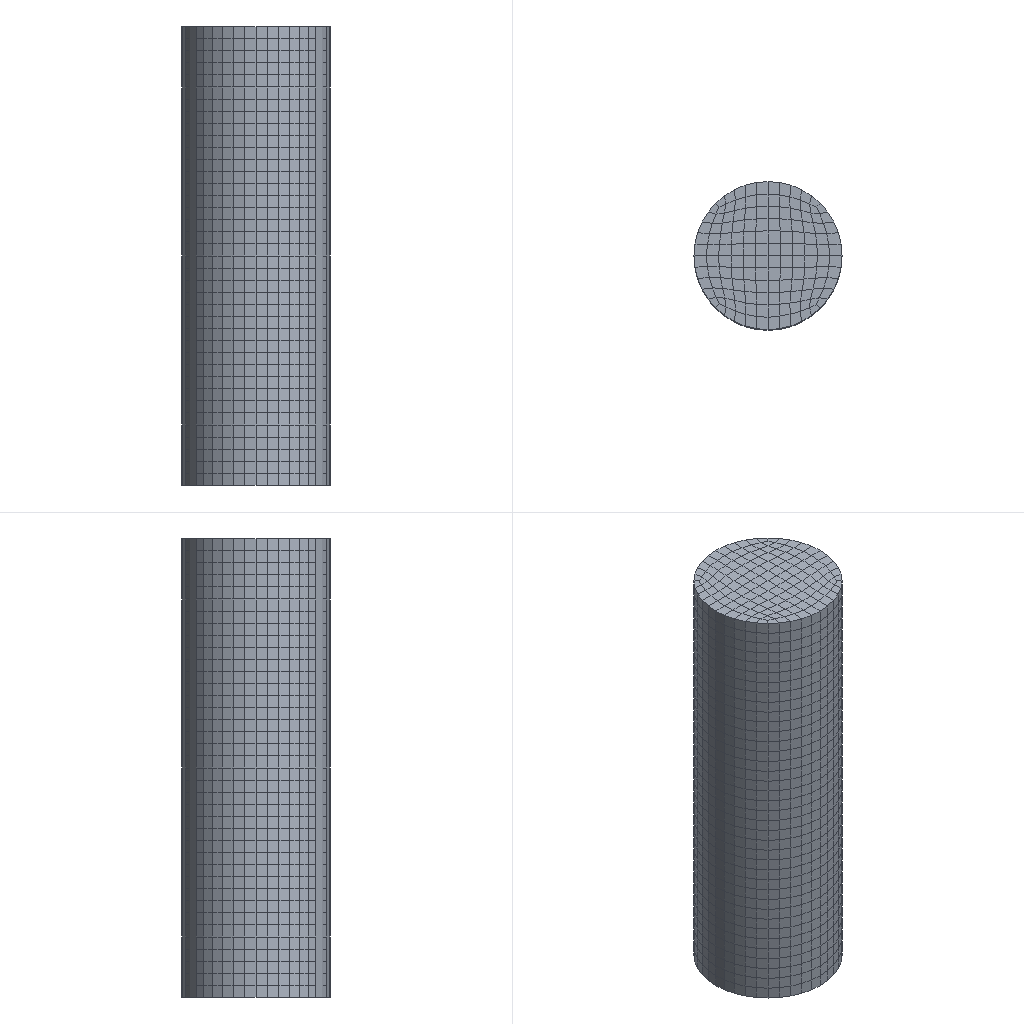Simulation study | abaqus
Set-up summary:
category,name,step,type,value,unit,region
solver,abaqus
solver,version,,,Abaqus/Standard 3DEXPERIENCE R2017x
units,not stated in the deck,,not stated
analysis,deck,,static,static
load_step,Step-1,Step-1,static,nlgeom=False
load_step,Step-2,Step-2,static,nlgeom=False
contact,interactions,,,general=0 pairs=1 ties=0
load_step,requested,,,2
mesh,nodes,,,7839
mesh,elements,,,6840
element_type,S4R,,shell,1520
element_type,C3D8R,,solid,5320
load,load commands in deck,,count,1
bc,support commands in deck,,count,13
material,H,,in results
material,S,,in results
check,setup vs results,,match,"per instance, exact: element labels, types and connectivity; labels of the nodes the elements use; coordinates of those nodes at SINGLE_PRECISION in 1 of 2 instance(s)"
Abaqus input file, long lists of numbers shortened:
*Heading
** Job name: Job-10 Model name: Model-1-Copy-Copy
** Generated by: Abaqus/CAE 2017
*Preprint, echo=NO, model=NO, history=NO, contact=NO
**
** PARTS
**
*Part, name=h
*Node
      1,           0.,           0.,         0.75
      2,           0., -0.121,         0.75
** (6277 more lines like these left out)
*Element, type=C3D8R
   1,  518,  519, 2929, 2641,   11,   12,  309,  308
   2,  519,  520, 2930, 2929,   12,   13,  310,  309
** (5318 more lines like these left out)
*Nset, nset=_PickedSet5, internal, generate
    1,  6279,     1
*Elset, elset=_PickedSet5, internal, generate
    1,  5320,     1
** Section: h
*Solid Section, elset=_PickedSet5, material=h
,
*End Part
**
*Part, name=ke
*Node
      1,           0., -0.121,           0.
      2,           0., -0.121,         0.75
** (1558 more lines like these left out)
*Element, type=S4R
  1,   1,   9, 229, 100
  2,   9,  10, 230, 229
** (1518 more lines like these left out)
*Nset, nset=Set-1, generate
    1,  1560,     1
*Elset, elset=Set-1, generate
    1,  1520,     1
** Section: Section-ke
*Shell Section, elset=Set-1, material=s, temperature=9, offset=-0.5
0.004, 9
*End Part
**
**
** ASSEMBLY
**
*Assembly, name=Assembly
**
*Instance, name=h-1, part=h
*End Instance
**
*Instance, name=ke-1, part=ke
*End Instance
**
*Node
      1,  -6.9388939e-18,  -7.40911299e-18,         0.75
*Node
      2,  2.08166817e-17,  -7.40911299e-18,           0.
*Nset, nset=Set-2, instance=h-1, generate
    1,  6279,     1
*Nset, nset=Set-2, instance=ke-1
 1, 2
*Elset, elset=Set-2, instance=h-1, generate
    1,  5320,     1
*Nset, nset=Set-3, instance=h-1, generate
    1,  6279,     1
*Nset, nset=Set-3, instance=ke-1, generate
    1,  1560,     1
*Elset, elset=Set-3, instance=h-1, generate
    1,  5320,     1
*Elset, elset=Set-3, instance=ke-1, generate
    1,  1520,     1
*Nset, nset=Set-4
 1,
*Nset, nset=Set-5
 2,
*Nset, nset=Set-9, instance=h-1, generate
    1,  6279,     1
*Nset, nset=Set-9, instance=ke-1, generate
    1,  1560,     1
*Elset, elset=Set-9, instance=h-1, generate
    1,  5320,     1
*Elset, elset=Set-9, instance=ke-1, generate
    1,  1520,     1
*Nset, nset=Set-10, instance=h-1, generate
    1,  6279,     1
*Nset, nset=Set-10, instance=ke-1, generate
    1,  1560,     1
*Elset, elset=Set-10, instance=h-1, generate
    1,  5320,     1
*Elset, elset=Set-10, instance=ke-1, generate
    1,  1520,     1
*Nset, nset=Set-11, instance=h-1, generate
    1,  6279,     1
*Nset, nset=Set-11, instance=ke-1, generate
    1,  1560,     1
*Elset, elset=Set-11, instance=h-1, generate
    1,  5320,     1
*Elset, elset=Set-11, instance=ke-1, generate
    1,  1520,     1
*Nset, nset=Set-19, instance=h-1, generate
    1,  6279,     1
*Nset, nset=Set-19, instance=ke-1, generate
    1,  1560,     1
*Elset, elset=Set-19, instance=h-1, generate
    1,  5320,     1
*Elset, elset=Set-19, instance=ke-1, generate
    1,  1520,     1
*Nset, nset=Set-20, instance=h-1
    1,    2,    3,    4,    5,    6,    7,    8,    9,   10,   11,   12,   13,   14,   15,   16
   17,   18,   19,   20,   21,   22,   23,   24,   25,   26,   27,   28,   29,   30,   31,   32
** (59 more lines like these left out)
*Nset, nset=Set-20, instance=ke-1, generate
    1,  1560,     1
*Elset, elset=Set-20, instance=h-1
    1,    2,    3,    4,    5,   10,   15,   20,   25,   26,   27,   28,   29,   30,   35,   40
   45,   50,   51,   52,   53,   54,   55,   60,   65,   70,   75,   76,   77,   78,   79,   80
** (103 more lines like these left out)
*Elset, elset=Set-20, instance=ke-1, generate
    1,  1520,     1
*Nset, nset=Set-21, instance=h-1
    1,    2,    3,    4,    5,    6,    7,    8,    9,   10,   11,   12,   13,   14,   15,   16
   17,   18,   19,   20,   21,   22,   23,   24,   25,   26,   27,   28,   29,   30,   31,   32
** (64 more lines like these left out)
*Elset, elset=Set-21, instance=h-1
    1,    2,    3,    4,    5,   10,   15,   20,   25,   26,   27,   28,   29,   30,   35,   40
   45,   50,   51,   52,   53,   54,   55,   60,   65,   70,   75,   76,   77,   78,   79,   80
** (107 more lines like these left out)
*Nset, nset=Set-22, instance=h-1, generate
    1,  6279,     1
*Nset, nset=Set-22, instance=ke-1, generate
    1,  1560,     1
*Elset, elset=Set-22, instance=h-1, generate
    1,  5320,     1
*Elset, elset=Set-22, instance=ke-1, generate
    1,  1520,     1
*Nset, nset=Set-23, instance=h-1, generate
    1,  6279,     1
*Elset, elset=Set-23, instance=h-1, generate
    1,  5320,     1
*Nset, nset=Set-24, instance=h-1
    1,    2,    3,    4,    5,    6,    7,    8,    9,   10,   11,   12,   13,   14,   15,   16
   17,   18,   19,   20,   21,   22,   23,   24,   25,   26,   27,   28,   29,   30,   31,   32
** (64 more lines like these left out)
*Elset, elset=Set-24, instance=h-1
    1,    2,    3,    4,    5,   10,   15,   20,   25,   26,   27,   28,   29,   30,   35,   40
   45,   50,   51,   52,   53,   54,   55,   60,   65,   70,   75,   76,   77,   78,   79,   80
** (107 more lines like these left out)
*Nset, nset=Set-25, instance=h-1, generate
    1,  6279,     1
*Elset, elset=Set-25, instance=h-1, generate
    1,  5320,     1
*Nset, nset=Set-26, instance=h-1
    1,    2,    3,    4,    5,    6,    7,    8,    9,   10,   11,   12,   13,   14,   15,   16
   17,   18,   19,   20,   21,   22,   23,   24,   25,   26,   27,   28,   29,   30,   31,   32
** (64 more lines like these left out)
*Nset, nset=Set-26, instance=ke-1, generate
    1,  1560,     1
*Elset, elset=Set-26, instance=h-1
    1,    2,    3,    4,    5,   10,   15,   20,   25,   26,   27,   28,   29,   30,   35,   40
   45,   50,   51,   52,   53,   54,   55,   60,   65,   70,   75,   76,   77,   78,   79,   80
** (107 more lines like these left out)
*Elset, elset=Set-26, instance=ke-1, generate
    1,  1520,     1
*Nset, nset=Set-27, instance=h-1, generate
    1,  6279,     1
*Elset, elset=Set-27, instance=h-1, generate
    1,  5320,     1
*Nset, nset=Set-28, instance=h-1, generate
    1,  6279,     1
*Elset, elset=Set-28, instance=h-1, generate
    1,  5320,     1
*Nset, nset=Set-29, instance=h-1
    1,    2,    3,    4,    5,    6,    7,    8,    9,   10,   11,   12,   13,   14,   15,   16
   17,   18,   19,   20,   21,   22,   23,   24,   25,   26,   27,   28,   29,   30,   31,   32
** (147 more lines like these left out)
*Elset, elset=Set-29, instance=h-1
    1,    2,    3,    4,    5,   10,   15,   20,   25,   26,   27,   28,   29,   30,   35,   40
   45,   50,   51,   52,   53,   54,   55,   60,   65,   70,   75,   76,   77,   78,   79,   80
** (179 more lines like these left out)
*Nset, nset=Set-30, instance=h-1, generate
    1,  6279,     1
*Nset, nset=Set-30, instance=ke-1, generate
    1,  1560,     1
*Elset, elset=Set-30, instance=h-1, generate
    1,  5320,     1
*Elset, elset=Set-30, instance=ke-1, generate
    1,  1520,     1
*Nset, nset=Set-31, instance=h-1, generate
    1,  6279,     1
*Nset, nset=Set-31, instance=ke-1, generate
    1,  1560,     1
*Elset, elset=Set-31, instance=h-1, generate
    1,  5320,     1
*Elset, elset=Set-31, instance=ke-1, generate
    1,  1520,     1
*Nset, nset=Set-32, instance=h-1
    1,    2,    3,    4,    5,    6,    7,    8,    9,   10,   11,   12,   13,   14,   15,   16
   17,   18,   19,   20,   21,   22,   23,   24,   25,   26,   27,   28,   29,   30,   31,   32
** (146 more lines like these left out)
*Nset, nset=Set-32, instance=ke-1, generate
    1,  1560,     1
*Elset, elset=Set-32, instance=h-1
    1,    2,    3,    4,    5,   10,   15,   20,   25,   26,   27,   28,   29,   30,   35,   40
   45,   50,   51,   52,   53,   54,   55,   60,   65,   70,   75,   76,   77,   78,   79,   80
** (163 more lines like these left out)
*Elset, elset=Set-32, instance=ke-1, generate
    1,  1520,     1
*Nset, nset=Set-33, instance=h-1, generate
    1,  6279,     1
*Elset, elset=Set-33, instance=h-1, generate
    1,  5320,     1
*Nset, nset=Set-37, instance=h-1, generate
    1,  6279,     1
*Elset, elset=Set-37, instance=h-1, generate
    1,  5320,     1
*Nset, nset=Set-38, instance=h-1, generate
    1,  6279,     1
*Elset, elset=Set-38, instance=h-1, generate
    1,  5320,     1
*Nset, nset=Set-39, instance=h-1, generate
    1,  6279,     1
*Nset, nset=Set-39, instance=ke-1, generate
    1,  1560,     1
*Elset, elset=Set-39, instance=h-1, generate
    1,  5320,     1
*Elset, elset=Set-39, instance=ke-1, generate
    1,  1520,     1
*Nset, nset=all, instance=h-1
    1,    2,    3,    4,    5,    6,    7,    8,    9,   10,   11,   12,   13,   14,   15,   16
   17,   18,   19,   20,   21,   22,   23,   24,   25,   26,   27,   28,   29,   30,   31,   32
** (147 more lines like these left out)
*Nset, nset=all, instance=ke-1, generate
    1,  1560,     1
*Elset, elset=all, instance=h-1
    1,    2,    3,    4,    5,   10,   15,   20,   25,   26,   27,   28,   29,   30,   35,   40
   45,   50,   51,   52,   53,   54,   55,   60,   65,   70,   75,   76,   77,   78,   79,   80
** (179 more lines like these left out)
*Elset, elset=all, instance=ke-1, generate
    1,  1520,     1
*Nset, nset=r1, instance=h-1
    1,    2,    3,    8,   10,   11,   12,   13,   14,   15,   16,   17,   18,   19,   20,   58
   59,   60,   61,   62,   63,   64,   65,   66,  211,  212,  213,  214,  215,  216,  217,  218
** (9 more lines like these left out)
*Nset, nset=r1, instance=ke-1
   2,   3,   5,   8,  46,  47,  48,  49,  50,  51,  52,  53,  54, 147, 148, 149
 150, 151, 152, 153, 154, 155, 202, 203, 204, 205, 206, 207, 208, 209, 210, 211
** (1 more lines like these left out)
*Nset, nset=r2, instance=h-1
    4,    5,    6,    7,    9,  141,  142,  143,  144,  145,  146,  147,  148,  149,  150,  151
  152,  153,  154,  155,  156,  157,  158,  159,  160,  161,  162,  163,  164,  165,  166,  167
** (9 more lines like these left out)
*Nset, nset=r2, instance=ke-1
   1,   4,   6,   7,  92,  93,  94,  95,  96,  97,  98,  99, 100, 138, 139, 140
 141, 142, 143, 144, 145, 146, 156, 157, 158, 159, 160, 161, 162, 163, 164, 220
** (1 more lines like these left out)
*Nset, nset=t_Set-5, instance=h-1
    1,    2,    3,    8,   10,   11,   12,   13,   14,   15,   16,   17,   18,   19,   20,   58
   59,   60,   61,   62,   63,   64,   65,   66,  211,  212,  213,  214,  215,  216,  217,  218
** (9 more lines like these left out)
*Nset, nset=t_Set-5, instance=ke-1
   2,   3,   5,   8,  46,  47,  48,  49,  50,  51,  52,  53,  54, 147, 148, 149
 150, 151, 152, 153, 154, 155, 202, 203, 204, 205, 206, 207, 208, 209, 210, 211
** (1 more lines like these left out)
*Elset, elset=t_Set-5, instance=h-1
    1,    2,    3,    4,    5,    6,    7,    8,    9,   10,   11,   12,   13,   14,   15,   16
   17,   18,   19,   20,   21,   22,   23,   24,   25,  476,  477,  478,  479,  480,  571,  572
** (7 more lines like these left out)
*Elset, elset=t_Set-5, instance=ke-1
   38,   76,  114,  152,  190,  228,  266,  304,  342,  380,  381,  419,  457,  495,  533,  571
  609,  647,  685,  723,  761,  799,  837,  875,  913,  951,  989, 1027, 1065, 1103, 1178, 1216
** (1 more lines like these left out)
*Nset, nset=t_Set-7, instance=h-1
    4,    5,    6,    7,    9,  141,  142,  143,  144,  145,  146,  147,  148,  149,  150,  151
  152,  153,  154,  155,  156,  157,  158,  159,  160,  161,  162,  163,  164,  165,  166,  167
** (9 more lines like these left out)
*Nset, nset=t_Set-7, instance=ke-1
   1,   4,   6,   7,  92,  93,  94,  95,  96,  97,  98,  99, 100, 138, 139, 140
 141, 142, 143, 144, 145, 146, 156, 157, 158, 159, 160, 161, 162, 163, 164, 220
** (1 more lines like these left out)
*Elset, elset=t_Set-7, instance=h-1
  684,  703,  722,  741,  760,  779,  798,  817,  836,  855,  874,  893,  912,  931,  950,  969
  988, 1007, 1026, 1045, 1064, 1083, 1102, 1121, 1140, 1141, 1160, 1179, 1198, 1217, 1254, 1273
** (7 more lines like these left out)
*Elset, elset=t_Set-7, instance=ke-1
    1,   39,   77,  115,  153,  191,  229,  267,  305,  343,  418,  456,  494,  532,  570,  608
  646,  684,  722,  760,  798,  836,  874,  912,  950,  988, 1026, 1064, 1102, 1140, 1141, 1179
** (1 more lines like these left out)
*Nset, nset=t_Set-12, instance=h-1
    1,    2,    3,    8,   10,   11,   12,   13,   14,   15,   16,   17,   18,   19,   20,   58
   59,   60,   61,   62,   63,   64,   65,   66,  211,  212,  213,  214,  215,  216,  217,  218
** (9 more lines like these left out)
*Nset, nset=t_Set-12
 1,
*Nset, nset=t_Set-12, instance=ke-1
   2,   3,   5,   8,  46,  47,  48,  49,  50,  51,  52,  53,  54, 147, 148, 149
 150, 151, 152, 153, 154, 155, 202, 203, 204, 205, 206, 207, 208, 209, 210, 211
** (1 more lines like these left out)
*Elset, elset=t_Set-12, instance=h-1
    1,    2,    3,    4,    5,    6,    7,    8,    9,   10,   11,   12,   13,   14,   15,   16
   17,   18,   19,   20,   21,   22,   23,   24,   25,  476,  477,  478,  479,  480,  571,  572
** (7 more lines like these left out)
*Elset, elset=t_Set-12, instance=ke-1
   38,   76,  114,  152,  190,  228,  266,  304,  342,  380,  381,  419,  457,  495,  533,  571
  609,  647,  685,  723,  761,  799,  837,  875,  913,  951,  989, 1027, 1065, 1103, 1178, 1216
** (1 more lines like these left out)
*Nset, nset=t_Set-13, instance=h-1
    4,    5,    6,    7,    9,  141,  142,  143,  144,  145,  146,  147,  148,  149,  150,  151
  152,  153,  154,  155,  156,  157,  158,  159,  160,  161,  162,  163,  164,  165,  166,  167
** (9 more lines like these left out)
*Nset, nset=t_Set-13
 2,
*Nset, nset=t_Set-13, instance=ke-1
   1,   4,   6,   7,  92,  93,  94,  95,  96,  97,  98,  99, 100, 138, 139, 140
 141, 142, 143, 144, 145, 146, 156, 157, 158, 159, 160, 161, 162, 163, 164, 220
** (1 more lines like these left out)
*Elset, elset=t_Set-13, instance=h-1
  684,  703,  722,  741,  760,  779,  798,  817,  836,  855,  874,  893,  912,  931,  950,  969
  988, 1007, 1026, 1045, 1064, 1083, 1102, 1121, 1140, 1141, 1160, 1179, 1198, 1217, 1254, 1273
** (7 more lines like these left out)
*Elset, elset=t_Set-13, instance=ke-1
    1,   39,   77,  115,  153,  191,  229,  267,  305,  343,  418,  456,  494,  532,  570,  608
  646,  684,  722,  760,  798,  836,  874,  912,  950,  988, 1026, 1064, 1102, 1140, 1141, 1179
** (1 more lines like these left out)
*Nset, nset=t_Set-17, instance=h-1
    1,    2,    3,    8,   10,   11,   12,   13,   14,   15,   16,   17,   18,   19,   20,   58
   59,   60,   61,   62,   63,   64,   65,   66,  211,  212,  213,  214,  215,  216,  217,  218
** (9 more lines like these left out)
*Nset, nset=t_Set-17, instance=ke-1
   2,   3,   5,   8,  46,  47,  48,  49,  50,  51,  52,  53,  54, 147, 148, 149
 150, 151, 152, 153, 154, 155, 202, 203, 204, 205, 206, 207, 208, 209, 210, 211
** (1 more lines like these left out)
*Elset, elset=t_Set-17, instance=h-1
    1,    2,    3,    4,    5,    6,    7,    8,    9,   10,   11,   12,   13,   14,   15,   16
   17,   18,   19,   20,   21,   22,   23,   24,   25,  476,  477,  478,  479,  480,  571,  572
** (7 more lines like these left out)
*Elset, elset=t_Set-17, instance=ke-1
   38,   76,  114,  152,  190,  228,  266,  304,  342,  380,  381,  419,  457,  495,  533,  571
  609,  647,  685,  723,  761,  799,  837,  875,  913,  951,  989, 1027, 1065, 1103, 1178, 1216
** (1 more lines like these left out)
*Nset, nset=t_Set-18, instance=h-1
    4,    5,    6,    7,    9,  141,  142,  143,  144,  145,  146,  147,  148,  149,  150,  151
  152,  153,  154,  155,  156,  157,  158,  159,  160,  161,  162,  163,  164,  165,  166,  167
** (9 more lines like these left out)
*Nset, nset=t_Set-18, instance=ke-1
   1,   4,   6,   7,  92,  93,  94,  95,  96,  97,  98,  99, 100, 138, 139, 140
 141, 142, 143, 144, 145, 146, 156, 157, 158, 159, 160, 161, 162, 163, 164, 220
** (1 more lines like these left out)
*Elset, elset=t_Set-18, instance=h-1
  684,  703,  722,  741,  760,  779,  798,  817,  836,  855,  874,  893,  912,  931,  950,  969
  988, 1007, 1026, 1045, 1064, 1083, 1102, 1121, 1140, 1141, 1160, 1179, 1198, 1217, 1254, 1273
** (7 more lines like these left out)
*Elset, elset=t_Set-18, instance=ke-1
    1,   39,   77,  115,  153,  191,  229,  267,  305,  343,  418,  456,  494,  532,  570,  608
  646,  684,  722,  760,  798,  836,  874,  912,  950,  988, 1026, 1064, 1102, 1140, 1141, 1179
** (1 more lines like these left out)
*Nset, nset=t_Set-34, instance=h-1
    1,    2,    3,    8,   10,   11,   12,   13,   14,   15,   16,   17,   18,   19,   20,   58
   59,   60,   61,   62,   63,   64,   65,   66,  211,  212,  213,  214,  215,  216,  217,  218
** (9 more lines like these left out)
*Nset, nset=t_Set-34, instance=ke-1
   2,   3,   5,   8,  46,  47,  48,  49,  50,  51,  52,  53,  54, 147, 148, 149
 150, 151, 152, 153, 154, 155, 202, 203, 204, 205, 206, 207, 208, 209, 210, 211
** (1 more lines like these left out)
*Elset, elset=t_Set-34, instance=h-1
    1,    2,    3,    4,    5,    6,    7,    8,    9,   10,   11,   12,   13,   14,   15,   16
   17,   18,   19,   20,   21,   22,   23,   24,   25,  476,  477,  478,  479,  480,  571,  572
** (7 more lines like these left out)
*Elset, elset=t_Set-34, instance=ke-1
   38,   76,  114,  152,  190,  228,  266,  304,  342,  380,  381,  419,  457,  495,  533,  571
  609,  647,  685,  723,  761,  799,  837,  875,  913,  951,  989, 1027, 1065, 1103, 1178, 1216
** (1 more lines like these left out)
*Nset, nset=t_Set-35, instance=h-1
    1,    2,    3,    8,   10,   11,   12,   13,   14,   15,   16,   17,   18,   19,   20,   58
   59,   60,   61,   62,   63,   64,   65,   66,  211,  212,  213,  214,  215,  216,  217,  218
** (9 more lines like these left out)
*Nset, nset=t_Set-35, instance=ke-1
   2,   3,   5,   8,  46,  47,  48,  49,  50,  51,  52,  53,  54, 147, 148, 149
 150, 151, 152, 153, 154, 155, 202, 203, 204, 205, 206, 207, 208, 209, 210, 211
** (1 more lines like these left out)
*Elset, elset=t_Set-35, instance=h-1
    1,    2,    3,    4,    5,    6,    7,    8,    9,   10,   11,   12,   13,   14,   15,   16
   17,   18,   19,   20,   21,   22,   23,   24,   25,  476,  477,  478,  479,  480,  571,  572
** (7 more lines like these left out)
*Elset, elset=t_Set-35, instance=ke-1
   38,   76,  114,  152,  190,  228,  266,  304,  342,  380,  381,  419,  457,  495,  533,  571
  609,  647,  685,  723,  761,  799,  837,  875,  913,  951,  989, 1027, 1065, 1103, 1178, 1216
** (1 more lines like these left out)
*Nset, nset=t_Set-36, instance=h-1
    4,    5,    6,    7,    9,  141,  142,  143,  144,  145,  146,  147,  148,  149,  150,  151
  152,  153,  154,  155,  156,  157,  158,  159,  160,  161,  162,  163,  164,  165,  166,  167
** (9 more lines like these left out)
*Nset, nset=t_Set-36, instance=ke-1
   1,   4,   6,   7,  92,  93,  94,  95,  96,  97,  98,  99, 100, 138, 139, 140
 141, 142, 143, 144, 145, 146, 156, 157, 158, 159, 160, 161, 162, 163, 164, 220
** (1 more lines like these left out)
*Elset, elset=t_Set-36, instance=h-1
  684,  703,  722,  741,  760,  779,  798,  817,  836,  855,  874,  893,  912,  931,  950,  969
  988, 1007, 1026, 1045, 1064, 1083, 1102, 1121, 1140, 1141, 1160, 1179, 1198, 1217, 1254, 1273
** (7 more lines like these left out)
*Elset, elset=t_Set-36, instance=ke-1
    1,   39,   77,  115,  153,  191,  229,  267,  305,  343,  418,  456,  494,  532,  570,  608
  646,  684,  722,  760,  798,  836,  874,  912,  950,  988, 1026, 1064, 1102, 1140, 1141, 1179
** (1 more lines like these left out)
*Nset, nset=_PickedSet69, internal
 1,
*Nset, nset=_PickedSet71, internal
 2,
*Elset, elset=_Surf-12_SPOS, internal, instance=ke-1, generate
    1,  1520,     1
*Surface, type=ELEMENT, name=Surf-12
_Surf-12_SPOS, SPOS
*Elset, elset=_m_Surf-7_S3, internal, instance=h-1
  571,  572,  573,  574,  575,  576,  577,  578,  579,  580,  581,  582,  583,  584,  585,  586
  587,  588,  589,  590,  591,  592,  593,  594,  595,  596,  597,  598,  599,  600,  601,  602
** (40 more lines like these left out)
*Elset, elset=_m_Surf-7_S4, internal, instance=h-1
  476,  477,  478,  479,  480,  481,  482,  483,  484,  485,  486,  487,  488,  489,  490,  491
  492,  493,  494,  495,  496,  497,  498,  499,  500,  501,  502,  503,  504,  505,  506,  507
** (52 more lines like these left out)
*Surface, type=ELEMENT, name=m_Surf-7
_m_Surf-7_S3, S3
_m_Surf-7_S4, S4
*Elset, elset=_m_Surf-13_S3, internal, instance=h-1
  571,  572,  573,  574,  575,  576,  577,  578,  579,  580,  581,  582,  583,  584,  585,  586
  587,  588,  589,  590,  591,  592,  593,  594,  595,  596,  597,  598,  599,  600,  601,  602
** (40 more lines like these left out)
*Elset, elset=_m_Surf-13_S4, internal, instance=h-1
  476,  477,  478,  479,  480,  481,  482,  483,  484,  485,  486,  487,  488,  489,  490,  491
  492,  493,  494,  495,  496,  497,  498,  499,  500,  501,  502,  503,  504,  505,  506,  507
** (52 more lines like these left out)
*Surface, type=ELEMENT, name=m_Surf-13
_m_Surf-13_S3, S3
_m_Surf-13_S4, S4
*Elset, elset=_s_Surf-9_S3, internal, instance=h-1
  571,  572,  573,  574,  575,  576,  577,  578,  579,  580,  581,  582,  583,  584,  585,  586
  587,  588,  589,  590,  591,  592,  593,  594,  595,  596,  597,  598,  599,  600,  601,  602
** (40 more lines like these left out)
*Elset, elset=_s_Surf-9_S4, internal, instance=h-1
  476,  477,  478,  479,  480,  481,  482,  483,  484,  485,  486,  487,  488,  489,  490,  491
  492,  493,  494,  495,  496,  497,  498,  499,  500,  501,  502,  503,  504,  505,  506,  507
** (52 more lines like these left out)
*Surface, type=ELEMENT, name=s_Surf-9
_s_Surf-9_S3, S3
_s_Surf-9_S4, S4
*Elset, elset=_s_Surf-11_SNEG, internal, instance=ke-1, generate
    1,  1520,     1
*Surface, type=ELEMENT, name=s_Surf-11
_s_Surf-11_SNEG, SNEG
*Elset, elset=_s_Surf-13_SNEG, internal, instance=ke-1, generate
    1,  1520,     1
*Surface, type=ELEMENT, name=s_Surf-13
_s_Surf-13_SNEG, SNEG
** Constraint: Constraint-1
*Rigid Body, ref node=_PickedSet69, tie nset=t_Set-35
** Constraint: Constraint-2
*Rigid Body, ref node=_PickedSet71, tie nset=t_Set-36
*End Assembly
*Amplitude, name=Amp-1, time=TOTAL TIME
             0.,             20.,             30.,        261.145,             60.,        349.214,             90.,        404.31
           120.,        444.505,            150.,        476.166,            180.,        502.289,            210.,        524.527
           240.,        543.887,            270.,        561.03,            300.,        576.41,            330.,        590.358
           360.,        603.118,            390.,        614.875,            420.,        625.777,            450.,        635.939
           480.,        645.455,            510.,         654.403,            540.,        662.846,            570.,        670.839
           600.,        678.427,            630.,        685.649,            660.,        692.54,            690.,        699.127
           720.,        705.436,            750.,        711.491,            780.,        717.31,            810.,        722.912
           840.,        728.312,            870.,        733.524,            900.,         738.561,            930.,         743.434
           960.,        748.153,            990.,        752.729,           1020.,        757.169,           1050.,        761.481
          1080.,        765.672,           1110.,        769.749,           1140.,        773.719,           1170.,        777.585
          1200.,         781.355,           1230.,         785.032,           1260.,        788.621,           1290.,        792.126
          1320.,        795.551,           1350.,        798.899,           1380.,        802.174,           1410.,        805.379
          1440.,        808.517,           1470.,        811.591,           1500.,        814.603,           1530.,        817.555
          1560.,        820.451,           1590.,         823.291,           1620.,        826.079,           1650.,        828.815
          1680.,         831.503,           1710.,        834.143,           1740.,        836.738,           1770.,        839.288
          1800.,        841.796,           1830.,        836.587,           1860.,        831.379,           1890.,        826.17
          1920.,        820.962,           1950.,        815.753,           1980.,        810.545,           2010.,        805.336
          2040.,        800.128,           2070.,        794.919,           2100.,        789.711,           2130.,        784.502
          2160.,        779.294,           2190.,        774.085,           2220.,        768.877,           2250.,        763.668
          2280.,        758.46,           2310.,        753.251,           2340.,        748.043,           2370.,        742.834
          2400.,        737.626,           2430.,        732.417,           2460.,        727.209,           2490.,        722.
          2520.,        716.792,           2550.,        711.583,           2580.,        706.375,           2610.,        701.166
          2640.,        695.958,           2670.,        690.749,           2700.,        685.541,           2730.,        680.332
          2760.,        675.124,           2790.,        669.915,           2820.,        664.707,           2850.,        659.498
          2880.,        654.29,           2910.,        649.081,           2940.,        643.873,           2970.,        638.664
          3000.,        633.456,           3030.,        628.247,           3060.,        623.039,           3090.,        617.83
          3120.,        612.622,           3150.,        607.413,           3180.,        602.205,           3210.,        596.996
          3240.,        591.788,           3270.,        586.579,           3300.,        581.371,           3330.,        576.162
          3360.,        570.954,           3390.,        565.745,           3420.,        560.537,           3450.,        555.328
          3480.,        550.12,           3510.,        544.911,           3540.,        539.703,           3570.,        534.494
          3600.,        529.286,           3630.,        524.077,           3660.,        518.869,           3690.,        513.66
          3720.,        508.452,           3750.,        503.243,           3780.,        498.035,           3810.,        492.826
          3840.,        487.618,           3870.,        482.409,           3900.,        477.201,           3930.,        471.992
          3960.,        466.784,           3990.,        461.575,           4020.,        456.367,           4050.,        451.158
          4080.,        445.95,           4110.,        440.741,           4140.,        435.533,           4170.,        430.324
          4200.,        425.116,           4230.,        419.907,           4260.,        414.699,           4290.,        409.49
          4320.,        404.282,           4350.,        399.073,           4380.,        393.865,           4410.,        388.656
          4440.,        383.448,           4470.,        378.239,           4500.,        373.031,           4530.,        367.822
          4560.,        362.614,           4590.,        357.405,           4620.,        352.197,           4650.,        346.988
          4680.,        341.78,           4710.,        336.571,           4740.,        331.363,           4770.,        326.154
** (261 more lines like these left out)
*Amplitude, name=Amp-2
             0.,              0.,              1.,              1.
**
** MATERIALS
**
*Material, name=H
*Density
2350.,
*Depvar
      3,
*Elastic, dependencies=1
 2.97254e+10,  0.2, ,  20.
  2.4771e+10,  0.2, , 100.
 1.98008e+10,  0.2, , 200.
 1.54661e+10,  0.2, , 300.
 1.15509e+10,  0.2, , 400.
    7.66e+09,  0.2, , 500.
 4.19821e+09,  0.2, , 600.
 1.95849e+09,  0.2, , 700.
 8.59467e+08,  0.2, , 800.
 3.82407e+08,  0.2, , 900.
 1.78048e+08,  0.2, ,1000.
 8.74176e+07,  0.2, ,1100.
 4.51827e+07,  0.2, ,1200.
*Expansion, user
*User Defined Field
*Concrete Damaged Plasticity
36.,      0.1,     1.16, 0.6368,   0.0005
*Concrete Compression Hardening, dependencies=1
 1.43927e+07,          0., , ,         20.
  2.5574e+07, 0.0001575, , ,         20.
 3.35487e+07, 0.0003985, , ,         20.
 3.83219e+07,  0.0007475, , ,         20.
 3.98983e+07,  0.001204, , ,         20.
 3.95871e+07,   0.001725, , ,         20.
 3.88784e+07,  0.002259, , ,         20.
 3.79552e+07,  0.002801, , ,         20.
 3.69236e+07,  0.003346, , ,         20.
 3.58465e+07,  0.003894, , ,         20.
 3.47617e+07,  0.004441, , ,         20.
 3.36919e+07,  0.004989, , ,         20.
 3.26505e+07,  0.005536, , ,         20.
 3.16451e+07,  0.006082, , ,         20.
 3.06797e+07,  0.006627, , ,         20.
 2.97559e+07,  0.007171, , ,         20.
 2.88738e+07,  0.007713, , ,         20.
 2.80328e+07,  0.008255, , ,         20.
 2.72315e+07,  0.008795, , ,         20.
 2.64683e+07,  0.009335, , ,         20.
 2.57414e+07,   0.009873, , ,         20.
 2.50488e+07,   0.01041, , ,         20.
 2.43888e+07,   0.01095, , ,         20.
 2.37594e+07,   0.01148, , ,         20.
 2.31589e+07,   0.01202, , ,         20.
 2.25856e+07,   0.01255, , ,         20.
  2.2038e+07,   0.01309, , ,         20.
 2.15144e+07,   0.01362, , ,         20.
 2.10135e+07,   0.01415, , ,         20.
 2.05339e+07,   0.01469, , ,         20.
 2.00744e+07,   0.01522, , ,         20.
 1.96339e+07,   0.01575, , ,         20.
 1.92112e+07,   0.01628, , ,         20.
 1.88054e+07,   0.01681, , ,         20.
 1.80407e+07,   0.01787, , ,         20.
 1.73328e+07,   0.01893, , ,         20.
 1.66759e+07,   0.01999, , ,         20.
 1.60649e+07,   0.02105, , ,         20.
 1.54952e+07,   0.02211, , ,         20.
 1.49629e+07,   0.02317, , ,         20.
** (545 more lines like these left out)
*Concrete Tension Stiffening, dependencies=1
 4.00054e+06,          0., , ,         20.
  3.7343e+06, 0.0001345, , ,         20.
   3.468e+06, 0.000269, , ,         20.
 3.20164e+06, 0.0004035, , ,         20.
  2.9352e+06, 0.000538, , ,         20.
  2.6687e+06, 0.0006725, , ,         20.
 2.40213e+06, 0.0008069, , ,         20.
  2.1355e+06, 0.0009414, , ,         20.
 1.86879e+06,   0.001076, , ,         20.
 1.60202e+06,  0.00121, , ,         20.
 1.33519e+06,  0.001345, , ,         20.
 1.06828e+06,  0.001479, , ,         20.
     801313.,  0.001613, , ,         20.
     534276.,  0.001748, , ,         20.
     267171.,   0.001882, , ,         20.
          0.,  0.002016, , ,         20.
 4.00062e+06,          0., , ,        100.
 3.73448e+06, 0.0001614, , ,        100.
 3.46825e+06, 0.0003228, , ,        100.
 3.20194e+06, 0.0004842, , ,        100.
 2.93556e+06,  0.0006455, , ,        100.
 2.66909e+06, 0.0008069, , ,        100.
 2.40254e+06, 0.0009682, , ,        100.
 2.13592e+06,   0.00113, , ,        100.
 1.86921e+06,  0.001291, , ,        100.
 1.60242e+06,  0.001452, , ,        100.
 1.33555e+06,   0.001613, , ,        100.
  1.0686e+06,  0.001775, , ,        100.
     801571.,  0.001936, , ,        100.
     534461.,  0.002097, , ,        100.
     267271.,  0.002258, , ,        100.
          0.,  0.002419, , ,        100.
 3.99754e+06,          0., , ,        200.
 3.73174e+06, 0.0002017, , ,        200.
 3.46584e+06, 0.0004034, , ,        200.
 3.19984e+06, 0.0006051, , ,        200.
 2.93374e+06, 0.0008068, , ,        200.
 2.66754e+06,  0.001008, , ,        200.
 2.40124e+06,  0.00121, , ,        200.
 2.13483e+06,  0.001412, , ,        200.
** (168 more lines like these left out)
*Material, name=s
*Elastic
 1.948e+11, 0.3
*Plastic
 3.04347e+08,          0.
 3.04537e+08, 0.0006182
 3.04584e+08, 0.0007736
 3.04821e+08,   0.00155
 3.05295e+08,  0.003102
 3.05769e+08,  0.004651
 3.06243e+08,  0.006197
 3.06717e+08,  0.007741
 3.07191e+08,  0.009283
 3.07665e+08,   0.01082
 3.08139e+08,   0.01236
 3.08613e+08,   0.01389
 3.10035e+08,   0.01848
 3.10983e+08,   0.02153
 3.11931e+08,   0.02457
 3.12879e+08,   0.0276
 3.13828e+08,   0.03062
 3.14776e+08,   0.03363
 3.15724e+08,   0.03664
 3.18094e+08,   0.0441
 3.22834e+08,   0.05887
 3.32314e+08,   0.08776
 3.41795e+08,    0.1158
 3.51275e+08,    0.1432
**
** INTERACTION PROPERTIES
**
*Surface Interaction, name=IntProp-1
1.,
*Friction, slip tolerance=0.005, taumax=400000.
 0.3,
*Surface Behavior, pressure-overclosure=HARD
**
** PREDEFINED FIELDS
**
** Name: Predefined Field-1   Type: Temperature
*Initial Conditions, type=TEMPERATURE
Set-39, 20., 20., 20., 20., 20., 20., 20.,
20., 20.
**
** INTERACTIONS
**
** Interaction: Int-1
*Contact Pair, interaction=IntProp-1, type=SURFACE TO SURFACE, adjust=0.0
s_Surf-13, m_Surf-13
** ----------------------------------------------------------------
**
** STEP: Step-1
**
*Step, name=Step-1, nlgeom=NO, inc=1000
*Static
30., 12000., 0.0003, 120.
**
** BOUNDARY CONDITIONS
**
** Name: BC-1 Type: 位移/转角
*Boundary
Set-4, 1, 1
Set-4, 2, 2
Set-4, 4, 4
Set-4, 5, 5
Set-4, 6, 6
** Name: BC-2 Type: 对称/反对称/完全固定
*Boundary
Set-5, ENCASTRE
**
** PREDEFINED FIELDS
**
** Name: Predefined Field-3   Type: Temperature
*Temperature, file=D:\FireAndZhouya\model\Job-5.odb, bstep=2, binc=1, estep=2, einc=100000
**
** OUTPUT REQUESTS
**
*Restart, write, frequency=0
**
** FIELD OUTPUT: F-Output-2
**
*Output, field, variable=PRESELECT
*Output, history, frequency=0
*End Step
** ----------------------------------------------------------------
**
** STEP: Step-2
**
*Step, name=Step-2, nlgeom=NO, inc=1000
*Static
0.005, 1., 1e-05, 0.1
**
** BOUNDARY CONDITIONS
**
** Name: BC-1 Type: 位移/转角
*Boundary, op=NEW
Set-4, 1, 1
Set-4, 2, 2
Set-4, 3, 3, -0.02
Set-4, 4, 4
Set-4, 5, 5
Set-4, 6, 6
** Name: BC-2 Type: 对称/反对称/完全固定
*Boundary, op=NEW
Set-5, ENCASTRE
**
** OUTPUT REQUESTS
**
*Restart, write, frequency=0
**
** FIELD OUTPUT: F-Output-2
**
*Output, field, variable=PRESELECT
**
** HISTORY OUTPUT: H-Output-2
**
*Output, history
*Node Output, nset=Set-4
RF3, U3
**
** HISTORY OUTPUT: H-Output-1
**
*Node Output, nset=Set-5
RF3,
*End Step
Results summary:
result,step,,completed,increments=103 time=12000.0/12000.0
result,step,,completed,increments=20 time=1.0/1.0
result,analysis,,,static
result,last_loadstep,,,2
result,analysis steps,,count,2
result,primary field,,,"U, UR"
result,reaction total,,FX,0.000734,model units
result,reaction total,,FY,0.000282,model units
result,reaction total,,FZ,0.0,model units